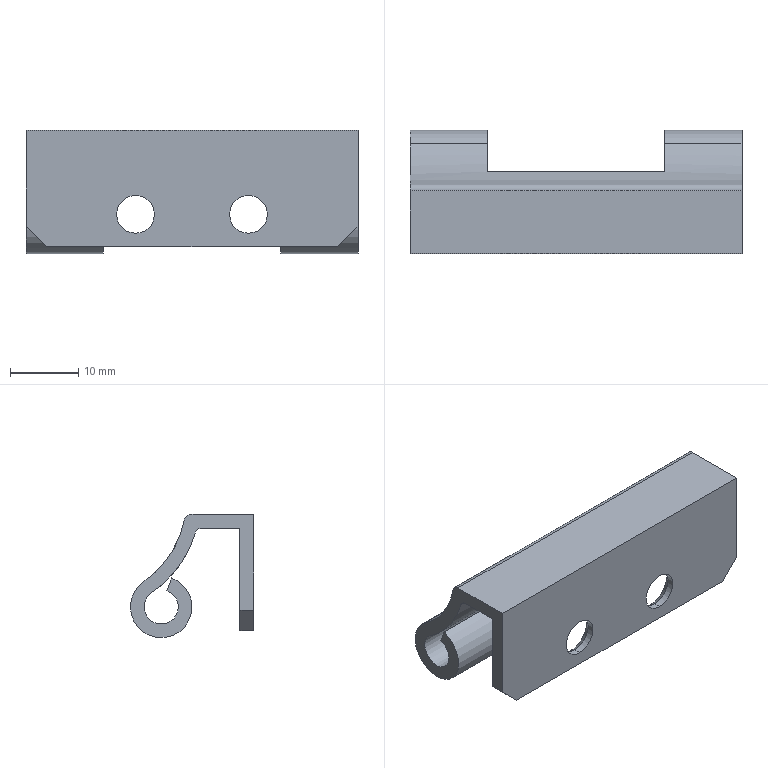Part | STEP file | 1 solid | 30 faces | box 48.5 x 18 x 18 mm | volume 3837 mm3 | plane 14 | cylinder 12 | cone 4 | commonest cylinder face diameters 5.5 x4 2 x2 5 x2 9 x2 28 x1 32 x1